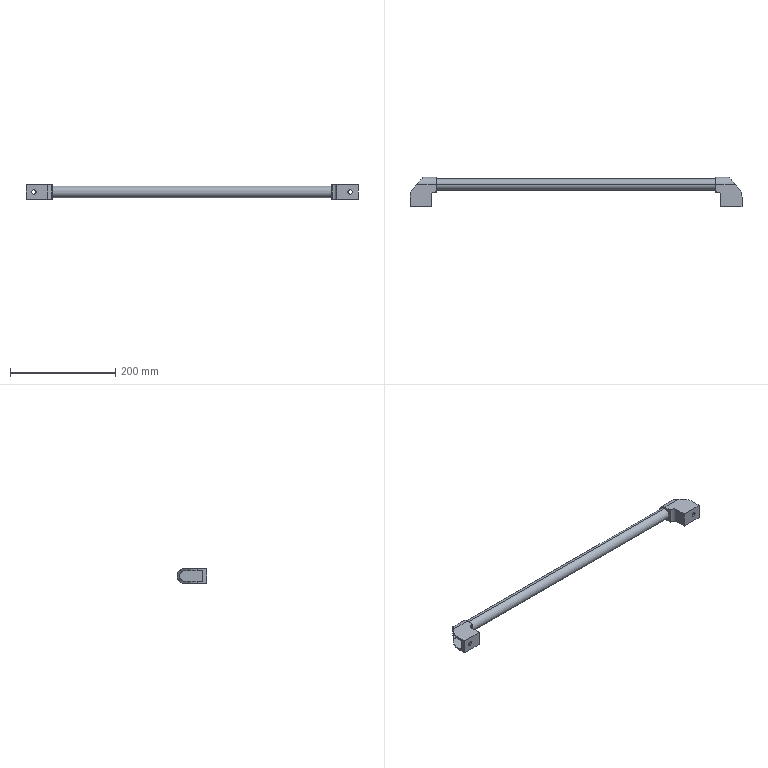Part | SolidWorks | features BaseBody 1 | 1 solid | 44 faces | box 630 x 56 x 28 mm | volume 285971 mm3 | plane 24 | cylinder 16 | cone 4 | commonest cylinder face diameters 8.2 x4 50 x4 16 x2 20 x2 22 x2 28 x2
STEP:
#1=CARTESIAN_POINT('',(265.,0.,11.));
#2=VERTEX_POINT('',#1);
#3=CARTESIAN_POINT('',(265.,0.,-11.));
#4=VERTEX_POINT('',#3);
#5=CARTESIAN_POINT('',(265.,0.,0.));
#6=DIRECTION('',(-1.,0.,0.));
#7=DIRECTION('',(0.,0.,1.));
#8=AXIS2_PLACEMENT_3D('',#5,#6,#7);
#9=CIRCLE('',#8,11.);
#10=EDGE_CURVE('',#2,#4,#9,.T.);
#11=ORIENTED_EDGE('',*,*,#10,.T.);
#12=CARTESIAN_POINT('',(-265.,0.,-11.));
#13=VERTEX_POINT('',#12);
#14=CARTESIAN_POINT('',(290.,0.,-11.));
#15=DIRECTION('',(-1.,0.,0.));
#16=VECTOR('',#15,1000.);
#17=LINE('',#14,#16);
#18=EDGE_CURVE('',#4,#13,#17,.T.);
#19=ORIENTED_EDGE('',*,*,#18,.T.);
#20=CARTESIAN_POINT('',(-265.,0.,11.));
#21=VERTEX_POINT('',#20);
#22=CARTESIAN_POINT('',(-265.,0.,0.));
#23=DIRECTION('',(1.,0.,0.));
#24=DIRECTION('',(0.,0.,1.));
#25=AXIS2_PLACEMENT_3D('',#22,#23,#24);
#26=CIRCLE('',#25,11.);
#27=EDGE_CURVE('',#13,#21,#26,.T.);
#28=ORIENTED_EDGE('',*,*,#27,.T.);
#29=CARTESIAN_POINT('',(290.,0.,11.));
#30=DIRECTION('',(-1.,0.,0.));
#31=VECTOR('',#30,1000.);
#32=LINE('',#29,#31);
#33=EDGE_CURVE('',#2,#21,#32,.T.);
#34=ORIENTED_EDGE('',*,*,#33,.F.);
#35=EDGE_LOOP('',(#11,#19,#28,#34));
#36=FACE_OUTER_BOUND('',#35,.T.);
#37=CARTESIAN_POINT('',(290.,0.,0.));
#38=DIRECTION('',(-1.,0.,0.));
#39=DIRECTION('',(0.,0.,1.));
#40=AXIS2_PLACEMENT_3D('',#37,#38,#39);
#41=CYLINDRICAL_SURFACE('',#40,11.);
#42=ADVANCED_FACE('',(#36),#41,.T.);
#43=CARTESIAN_POINT('',(-300.,-42.,4.1));
#44=VERTEX_POINT('',#43);
#45=CARTESIAN_POINT('',(-300.,-42.,-4.1));
#46=VERTEX_POINT('',#45);
#47=CARTESIAN_POINT('',(-300.,-42.,0.));
#48=DIRECTION('',(0.,-1.,0.));
#49=DIRECTION('',(0.,0.,1.));
#50=AXIS2_PLACEMENT_3D('',#47,#48,#49);
#51=CIRCLE('',#50,4.1);
#52=EDGE_CURVE('',#44,#46,#51,.T.);
#53=ORIENTED_EDGE('',*,*,#52,.T.);
#54=CARTESIAN_POINT('',(-300.,-38.,-4.1));
#55=VERTEX_POINT('',#54);
#56=CARTESIAN_POINT('',(-300.,-42.,-4.1));
#57=DIRECTION('',(0.,1.,0.));
#58=VECTOR('',#57,1000.);
#59=LINE('',#56,#58);
#60=EDGE_CURVE('',#46,#55,#59,.T.);
#61=ORIENTED_EDGE('',*,*,#60,.T.);
#62=CARTESIAN_POINT('',(-300.,-38.,4.1));
#63=VERTEX_POINT('',#62);
#64=CARTESIAN_POINT('',(-300.,-38.,0.));
#65=DIRECTION('',(0.,-1.,0.));
#66=DIRECTION('',(0.,0.,1.));
#67=AXIS2_PLACEMENT_3D('',#64,#65,#66);
#68=CIRCLE('',#67,4.1);
#69=EDGE_CURVE('',#63,#55,#68,.T.);
#70=ORIENTED_EDGE('',*,*,#69,.F.);
#71=CARTESIAN_POINT('',(-300.,-42.,4.1));
#72=DIRECTION('',(0.,1.,0.));
#73=VECTOR('',#72,1000.);
#74=LINE('',#71,#73);
#75=EDGE_CURVE('',#44,#63,#74,.T.);
#76=ORIENTED_EDGE('',*,*,#75,.F.);
#77=EDGE_LOOP('',(#53,#61,#70,#76));
#78=FACE_OUTER_BOUND('',#77,.T.);
#79=CARTESIAN_POINT('',(-300.,-42.,0.));
#80=DIRECTION('',(0.,1.,0.));
#81=DIRECTION('',(0.,0.,1.));
#82=AXIS2_PLACEMENT_3D('',#79,#80,#81);
#83=CYLINDRICAL_SURFACE('',#82,4.1);
#84=ADVANCED_FACE('',(#78),#83,.F.);
#85=CARTESIAN_POINT('',(300.,-42.,-4.1));
#86=VERTEX_POINT('',#85);
#87=CARTESIAN_POINT('',(300.,-42.,4.1));
#88=VERTEX_POINT('',#87);
#89=CARTESIAN_POINT('',(300.,-42.,0.));
#90=DIRECTION('',(0.,1.,0.));
#91=DIRECTION('',(0.,0.,1.));
#92=AXIS2_PLACEMENT_3D('',#89,#90,#91);
#93=CIRCLE('',#92,4.1);
#94=EDGE_CURVE('',#86,#88,#93,.T.);
#95=ORIENTED_EDGE('',*,*,#94,.F.);
#96=CARTESIAN_POINT('',(300.,-38.,-4.1));
#97=VERTEX_POINT('',#96);
#98=CARTESIAN_POINT('',(300.,-42.,-4.1));
#99=DIRECTION('',(0.,1.,0.));
#100=VECTOR('',#99,1000.);
#101=LINE('',#98,#100);
#102=EDGE_CURVE('',#86,#97,#101,.T.);
#103=ORIENTED_EDGE('',*,*,#102,.T.);
#104=CARTESIAN_POINT('',(300.,-38.,4.1));
#105=VERTEX_POINT('',#104);
#106=CARTESIAN_POINT('',(300.,-38.,0.));
#107=DIRECTION('',(0.,-1.,0.));
#108=DIRECTION('',(0.,0.,1.));
#109=AXIS2_PLACEMENT_3D('',#106,#107,#108);
#110=CIRCLE('',#109,4.1);
#111=EDGE_CURVE('',#105,#97,#110,.T.);
#112=ORIENTED_EDGE('',*,*,#111,.F.);
#113=CARTESIAN_POINT('',(300.,-42.,4.1));
#114=DIRECTION('',(0.,1.,0.));
#115=VECTOR('',#114,1000.);
#116=LINE('',#113,#115);
#117=EDGE_CURVE('',#88,#105,#116,.T.);
#118=ORIENTED_EDGE('',*,*,#117,.F.);
#119=EDGE_LOOP('',(#95,#103,#112,#118));
#120=FACE_OUTER_BOUND('',#119,.T.);
#121=CARTESIAN_POINT('',(300.,-42.,0.));
#122=DIRECTION('',(0.,1.,0.));
#123=DIRECTION('',(0.,0.,1.));
#124=AXIS2_PLACEMENT_3D('',#121,#122,#123);
#125=CYLINDRICAL_SURFACE('',#124,4.1);
#126=ADVANCED_FACE('',(#120),#125,.F.);
#127=ORIENTED_EDGE('',*,*,#69,.T.);
#128=CARTESIAN_POINT('',(-300.,-34.,-8.));
#129=VERTEX_POINT('',#128);
#130=CARTESIAN_POINT('',(-300.,-34.,-8.));
#131=DIRECTION('',(0.,0.716,-0.6981));
#132=VECTOR('',#131,1000.);
#133=LINE('',#130,#132);
#134=EDGE_CURVE('',#55,#129,#133,.T.);
#135=ORIENTED_EDGE('',*,*,#134,.T.);
#136=CARTESIAN_POINT('',(-300.,-34.,8.));
#137=VERTEX_POINT('',#136);
#138=CARTESIAN_POINT('',(-300.,-34.,0.));
#139=DIRECTION('',(0.,-1.,0.));
#140=DIRECTION('',(0.,0.,1.));
#141=AXIS2_PLACEMENT_3D('',#138,#139,#140);
#142=CIRCLE('',#141,8.);
#143=EDGE_CURVE('',#137,#129,#142,.T.);
#144=ORIENTED_EDGE('',*,*,#143,.F.);
#145=CARTESIAN_POINT('',(-300.,-34.,8.));
#146=DIRECTION('',(0.,0.716,0.6981));
#147=VECTOR('',#146,1000.);
#148=LINE('',#145,#147);
#149=EDGE_CURVE('',#63,#137,#148,.T.);
#150=ORIENTED_EDGE('',*,*,#149,.F.);
#151=EDGE_LOOP('',(#127,#135,#144,#150));
#152=FACE_OUTER_BOUND('',#151,.T.);
#153=CARTESIAN_POINT('',(-300.,-34.,0.));
#154=DIRECTION('',(0.,1.,0.));
#155=DIRECTION('',(0.,0.,1.));
#156=AXIS2_PLACEMENT_3D('',#153,#154,#155);
#157=CONICAL_SURFACE('',#156,8.,0.7727);
#158=ADVANCED_FACE('',(#152),#157,.F.);
#159=ORIENTED_EDGE('',*,*,#111,.T.);
#160=CARTESIAN_POINT('',(300.,-34.,-8.));
#161=VERTEX_POINT('',#160);
#162=CARTESIAN_POINT('',(300.,-34.,-8.));
#163=DIRECTION('',(0.,0.716,-0.6981));
#164=VECTOR('',#163,1000.);
#165=LINE('',#162,#164);
#166=EDGE_CURVE('',#97,#161,#165,.T.);
#167=ORIENTED_EDGE('',*,*,#166,.T.);
#168=CARTESIAN_POINT('',(300.,-34.,8.));
#169=VERTEX_POINT('',#168);
#170=CARTESIAN_POINT('',(300.,-34.,0.));
#171=DIRECTION('',(0.,1.,0.));
#172=DIRECTION('',(0.,0.,1.));
#173=AXIS2_PLACEMENT_3D('',#170,#171,#172);
#174=CIRCLE('',#173,8.);
#175=EDGE_CURVE('',#161,#169,#174,.T.);
#176=ORIENTED_EDGE('',*,*,#175,.T.);
#177=CARTESIAN_POINT('',(300.,-34.,8.));
#178=DIRECTION('',(0.,0.716,0.6981));
#179=VECTOR('',#178,1000.);
#180=LINE('',#177,#179);
#181=EDGE_CURVE('',#105,#169,#180,.T.);
#182=ORIENTED_EDGE('',*,*,#181,.F.);
#183=EDGE_LOOP('',(#159,#167,#176,#182));
#184=FACE_OUTER_BOUND('',#183,.T.);
#185=CARTESIAN_POINT('',(300.,-34.,0.));
#186=DIRECTION('',(0.,1.,0.));
#187=DIRECTION('',(0.,0.,1.));
#188=AXIS2_PLACEMENT_3D('',#185,#186,#187);
#189=CONICAL_SURFACE('',#188,8.,0.7727);
#190=ADVANCED_FACE('',(#184),#189,.F.);
#191=ORIENTED_EDGE('',*,*,#18,.F.);
#192=CARTESIAN_POINT('',(265.,0.,0.));
#193=DIRECTION('',(-1.,0.,0.));
#194=DIRECTION('',(0.,0.,1.));
#195=AXIS2_PLACEMENT_3D('',#192,#193,#194);
#196=CIRCLE('',#195,11.);
#197=EDGE_CURVE('',#4,#2,#196,.T.);
#198=ORIENTED_EDGE('',*,*,#197,.T.);
#199=ORIENTED_EDGE('',*,*,#33,.T.);
#200=CARTESIAN_POINT('',(-265.,0.,0.));
#201=DIRECTION('',(1.,0.,0.));
#202=DIRECTION('',(0.,0.,1.));
#203=AXIS2_PLACEMENT_3D('',#200,#201,#202);
#204=CIRCLE('',#203,11.);
#205=EDGE_CURVE('',#21,#13,#204,.T.);
#206=ORIENTED_EDGE('',*,*,#205,.T.);
#207=EDGE_LOOP('',(#191,#198,#199,#206));
#208=FACE_OUTER_BOUND('',#207,.T.);
#209=CARTESIAN_POINT('',(290.,0.,0.));
#210=DIRECTION('',(-1.,0.,0.));
#211=DIRECTION('',(0.,0.,1.));
#212=AXIS2_PLACEMENT_3D('',#209,#210,#211);
#213=CYLINDRICAL_SURFACE('',#212,11.);
#214=ADVANCED_FACE('',(#208),#213,.T.);
#215=ORIENTED_EDGE('',*,*,#205,.F.);
#216=ORIENTED_EDGE('',*,*,#27,.F.);
#217=EDGE_LOOP('',(#215,#216));
#218=FACE_BOUND('',#217,.T.);
#219=CARTESIAN_POINT('',(-265.,0.,-14.));
#220=VERTEX_POINT('',#219);
#221=CARTESIAN_POINT('',(-265.,-14.,-14.));
#222=VERTEX_POINT('',#221);
#223=CARTESIAN_POINT('',(-265.,-14.,-14.));
#224=DIRECTION('',(0.,-1.,0.));
#225=VECTOR('',#224,1000.);
#226=LINE('',#223,#225);
#227=EDGE_CURVE('',#220,#222,#226,.T.);
#228=ORIENTED_EDGE('',*,*,#227,.F.);
#229=CARTESIAN_POINT('',(-265.,0.000000104,14.));
#230=VERTEX_POINT('',#229);
#231=CARTESIAN_POINT('',(-265.,0.,0.));
#232=DIRECTION('',(-1.,0.,0.));
#233=DIRECTION('',(0.,0.,-1.));
#234=AXIS2_PLACEMENT_3D('',#231,#232,#233);
#235=CIRCLE('',#234,14.);
#236=EDGE_CURVE('',#230,#220,#235,.T.);
#237=ORIENTED_EDGE('',*,*,#236,.F.);
#238=CARTESIAN_POINT('',(-265.,-14.,14.));
#239=VERTEX_POINT('',#238);
#240=CARTESIAN_POINT('',(-265.,-14.,14.));
#241=DIRECTION('',(0.,1.,0.));
#242=VECTOR('',#241,1000.);
#243=LINE('',#240,#242);
#244=EDGE_CURVE('',#239,#230,#243,.T.);
#245=ORIENTED_EDGE('',*,*,#244,.F.);
#246=CARTESIAN_POINT('',(-265.,-14.,28.));
#247=DIRECTION('',(0.,0.,1.));
#248=VECTOR('',#247,1000.);
#249=LINE('',#246,#248);
#250=EDGE_CURVE('',#222,#239,#249,.T.);
#251=ORIENTED_EDGE('',*,*,#250,.F.);
#252=EDGE_LOOP('',(#228,#237,#245,#251));
#253=FACE_OUTER_BOUND('',#252,.T.);
#254=CARTESIAN_POINT('',(-265.,-14.,28.));
#255=DIRECTION('',(-1.,0.,0.));
#256=DIRECTION('',(0.,0.,1.));
#257=AXIS2_PLACEMENT_3D('',#254,#255,#256);
#258=PLANE('',#257);
#259=ADVANCED_FACE('',(#218,#253),#258,.F.);
#260=CARTESIAN_POINT('',(265.,0.000000104,14.));
#261=VERTEX_POINT('',#260);
#262=CARTESIAN_POINT('',(265.,-14.,14.));
#263=VERTEX_POINT('',#262);
#264=CARTESIAN_POINT('',(265.,0.,14.));
#265=DIRECTION('',(0.,-1.,0.));
#266=VECTOR('',#265,1000.);
#267=LINE('',#264,#266);
#268=EDGE_CURVE('',#261,#263,#267,.T.);
#269=ORIENTED_EDGE('',*,*,#268,.F.);
#270=CARTESIAN_POINT('',(265.,0.,-14.));
#271=VERTEX_POINT('',#270);
#272=CARTESIAN_POINT('',(265.,0.,0.));
#273=DIRECTION('',(1.,0.,0.));
#274=DIRECTION('',(0.,0.,1.));
#275=AXIS2_PLACEMENT_3D('',#272,#273,#274);
#276=CIRCLE('',#275,14.);
#277=EDGE_CURVE('',#271,#261,#276,.T.);
#278=ORIENTED_EDGE('',*,*,#277,.F.);
#279=CARTESIAN_POINT('',(265.,-14.,-14.));
#280=VERTEX_POINT('',#279);
#281=CARTESIAN_POINT('',(265.,0.,-14.));
#282=DIRECTION('',(0.,1.,0.));
#283=VECTOR('',#282,1000.);
#284=LINE('',#281,#283);
#285=EDGE_CURVE('',#280,#271,#284,.T.);
#286=ORIENTED_EDGE('',*,*,#285,.F.);
#287=CARTESIAN_POINT('',(265.,-14.,0.));
#288=DIRECTION('',(0.,0.,-1.));
#289=VECTOR('',#288,1000.);
#290=LINE('',#287,#289);
#291=EDGE_CURVE('',#263,#280,#290,.T.);
#292=ORIENTED_EDGE('',*,*,#291,.F.);
#293=EDGE_LOOP('',(#269,#278,#286,#292));
#294=FACE_OUTER_BOUND('',#293,.T.);
#295=ORIENTED_EDGE('',*,*,#10,.F.);
#296=ORIENTED_EDGE('',*,*,#197,.F.);
#297=EDGE_LOOP('',(#295,#296));
#298=FACE_BOUND('',#297,.T.);
#299=CARTESIAN_POINT('',(265.,0.,0.));
#300=DIRECTION('',(1.,0.,0.));
#301=DIRECTION('',(0.,0.,-1.));
#302=AXIS2_PLACEMENT_3D('',#299,#300,#301);
#303=PLANE('',#302);
#304=ADVANCED_FACE('',(#294,#298),#303,.F.);
#305=CARTESIAN_POINT('',(-267.,-14.,-14.));
#306=VERTEX_POINT('',#305);
#307=CARTESIAN_POINT('',(-267.,-14.,-14.));
#308=DIRECTION('',(-1.,0.,0.));
#309=VECTOR('',#308,1000.);
#310=LINE('',#307,#309);
#311=EDGE_CURVE('',#222,#306,#310,.T.);
#312=ORIENTED_EDGE('',*,*,#311,.F.);
#313=ORIENTED_EDGE('',*,*,#250,.T.);
#314=CARTESIAN_POINT('',(-267.,-14.,14.));
#315=VERTEX_POINT('',#314);
#316=CARTESIAN_POINT('',(-267.,-14.,14.));
#317=DIRECTION('',(1.,0.,0.));
#318=VECTOR('',#317,1000.);
#319=LINE('',#316,#318);
#320=EDGE_CURVE('',#315,#239,#319,.T.);
#321=ORIENTED_EDGE('',*,*,#320,.F.);
#322=CARTESIAN_POINT('',(-267.,-14.,28.));
#323=DIRECTION('',(0.,0.,1.));
#324=VECTOR('',#323,1000.);
#325=LINE('',#322,#324);
#326=EDGE_CURVE('',#306,#315,#325,.T.);
#327=ORIENTED_EDGE('',*,*,#326,.F.);
#328=EDGE_LOOP('',(#312,#313,#321,#327));
#329=FACE_OUTER_BOUND('',#328,.T.);
#330=CARTESIAN_POINT('',(-267.,-14.,28.));
#331=DIRECTION('',(0.,1.,0.));
#332=DIRECTION('',(0.,0.,1.));
#333=AXIS2_PLACEMENT_3D('',#330,#331,#332);
#334=PLANE('',#333);
#335=ADVANCED_FACE('',(#329),#334,.F.);
#336=CARTESIAN_POINT('',(-308.648,-6.886,-14.));
#337=VERTEX_POINT('',#336);
#338=CARTESIAN_POINT('',(-315.,-23.537,-14.));
#339=VERTEX_POINT('',#338);
#340=CARTESIAN_POINT('',(-290.,-23.537,-14.));
#341=DIRECTION('',(0.,0.,1.));
#342=DIRECTION('',(1.,0.,0.));
#343=AXIS2_PLACEMENT_3D('',#340,#341,#342);
#344=CIRCLE('',#343,25.);
#345=EDGE_CURVE('',#337,#339,#344,.T.);
#346=ORIENTED_EDGE('',*,*,#345,.F.);
#347=CARTESIAN_POINT('',(-302.5,0.,-14.));
#348=VERTEX_POINT('',#347);
#349=CARTESIAN_POINT('',(-302.5,0.,-14.));
#350=DIRECTION('',(-0.666,-0.7459,0.));
#351=VECTOR('',#350,1000.);
#352=LINE('',#349,#351);
#353=EDGE_CURVE('',#348,#337,#352,.T.);
#354=ORIENTED_EDGE('',*,*,#353,.F.);
#355=CARTESIAN_POINT('',(315.,0.,-14.));
#356=DIRECTION('',(-1.,0.,0.));
#357=VECTOR('',#356,1000.);
#358=LINE('',#355,#357);
#359=EDGE_CURVE('',#220,#348,#358,.T.);
#360=ORIENTED_EDGE('',*,*,#359,.F.);
#361=ORIENTED_EDGE('',*,*,#227,.T.);
#362=ORIENTED_EDGE('',*,*,#311,.T.);
#363=CARTESIAN_POINT('',(-275.,-22.,-14.));
#364=VERTEX_POINT('',#363);
#365=CARTESIAN_POINT('',(-267.,-22.,-14.));
#366=DIRECTION('',(0.,0.,-1.));
#367=DIRECTION('',(1.,0.,0.));
#368=AXIS2_PLACEMENT_3D('',#365,#366,#367);
#369=CIRCLE('',#368,8.);
#370=EDGE_CURVE('',#364,#306,#369,.T.);
#371=ORIENTED_EDGE('',*,*,#370,.F.);
#372=CARTESIAN_POINT('',(-275.,-42.,-14.));
#373=VERTEX_POINT('',#372);
#374=CARTESIAN_POINT('',(-275.,-42.,-14.));
#375=DIRECTION('',(0.,1.,0.));
#376=VECTOR('',#375,1000.);
#377=LINE('',#374,#376);
#378=EDGE_CURVE('',#373,#364,#377,.T.);
#379=ORIENTED_EDGE('',*,*,#378,.F.);
#380=CARTESIAN_POINT('',(-315.,-42.,-14.));
#381=VERTEX_POINT('',#380);
#382=CARTESIAN_POINT('',(315.,-42.,-14.));
#383=DIRECTION('',(1.,0.,0.));
#384=VECTOR('',#383,1000.);
#385=LINE('',#382,#384);
#386=EDGE_CURVE('',#381,#373,#385,.T.);
#387=ORIENTED_EDGE('',*,*,#386,.F.);
#388=CARTESIAN_POINT('',(-315.,-42.,-14.));
#389=DIRECTION('',(0.,-1.,0.));
#390=VECTOR('',#389,1000.);
#391=LINE('',#388,#390);
#392=EDGE_CURVE('',#339,#381,#391,.T.);
#393=ORIENTED_EDGE('',*,*,#392,.F.);
#394=EDGE_LOOP('',(#346,#354,#360,#361,#362,#371,#379,#387,#393));
#395=FACE_OUTER_BOUND('',#394,.T.);
#396=CARTESIAN_POINT('',(315.,-42.,-14.));
#397=DIRECTION('',(0.,0.,1.));
#398=DIRECTION('',(1.,0.,0.));
#399=AXIS2_PLACEMENT_3D('',#396,#397,#398);
#400=PLANE('',#399);
#401=ADVANCED_FACE('',(#395),#400,.F.);
#402=CARTESIAN_POINT('',(-302.5,0.000000104,14.));
#403=VERTEX_POINT('',#402);
#404=CARTESIAN_POINT('',(-302.5,0.,-14.));
#405=CARTESIAN_POINT('',(-277.5,28.,-14.));
#406=CARTESIAN_POINT('',(-277.5,28.,14.));
#407=CARTESIAN_POINT('',(-302.5,0.000000104,14.));
#408=(BOUNDED_CURVE()B_SPLINE_CURVE(3,(#404,#405,#406,#407),.UNSPECIFIED.,.F.,.T.)B_SPLINE_CURVE_WITH_KNOTS((4,4),(4.712,7.854),.UNSPECIFIED.)CURVE()GEOMETRIC_REPRESENTATION_ITEM()RATIONAL_B_SPLINE_CURVE((1.,0.3333,0.3333,1.))REPRESENTATION_ITEM(''));
#409=EDGE_CURVE('',#348,#403,#408,.T.);
#410=ORIENTED_EDGE('',*,*,#409,.T.);
#411=CARTESIAN_POINT('',(315.,0.000000209,14.));
#412=DIRECTION('',(1.,0.,0.));
#413=VECTOR('',#412,1000.);
#414=LINE('',#411,#413);
#415=EDGE_CURVE('',#403,#230,#414,.T.);
#416=ORIENTED_EDGE('',*,*,#415,.T.);
#417=ORIENTED_EDGE('',*,*,#236,.T.);
#418=ORIENTED_EDGE('',*,*,#359,.T.);
#419=EDGE_LOOP('',(#410,#416,#417,#418));
#420=FACE_OUTER_BOUND('',#419,.T.);
#421=CARTESIAN_POINT('',(315.,0.,0.));
#422=DIRECTION('',(1.,0.,0.));
#423=DIRECTION('',(0.,0.,-1.));
#424=AXIS2_PLACEMENT_3D('',#421,#422,#423);
#425=CYLINDRICAL_SURFACE('',#424,14.);
#426=ADVANCED_FACE('',(#420),#425,.T.);
#427=CARTESIAN_POINT('',(-315.,-23.537,14.));
#428=VERTEX_POINT('',#427);
#429=CARTESIAN_POINT('',(-308.648,-6.886,14.));
#430=VERTEX_POINT('',#429);
#431=CARTESIAN_POINT('',(-290.,-23.537,14.));
#432=DIRECTION('',(0.,0.,-1.));
#433=DIRECTION('',(1.,0.,0.));
#434=AXIS2_PLACEMENT_3D('',#431,#432,#433);
#435=CIRCLE('',#434,25.);
#436=EDGE_CURVE('',#428,#430,#435,.T.);
#437=ORIENTED_EDGE('',*,*,#436,.F.);
#438=CARTESIAN_POINT('',(-315.,-42.,14.));
#439=VERTEX_POINT('',#438);
#440=CARTESIAN_POINT('',(-315.,0.,14.));
#441=DIRECTION('',(0.,1.,0.));
#442=VECTOR('',#441,1000.);
#443=LINE('',#440,#442);
#444=EDGE_CURVE('',#439,#428,#443,.T.);
#445=ORIENTED_EDGE('',*,*,#444,.F.);
#446=CARTESIAN_POINT('',(-275.,-42.,14.));
#447=VERTEX_POINT('',#446);
#448=CARTESIAN_POINT('',(315.,-42.,14.));
#449=DIRECTION('',(-1.,0.,0.));
#450=VECTOR('',#449,1000.);
#451=LINE('',#448,#450);
#452=EDGE_CURVE('',#447,#439,#451,.T.);
#453=ORIENTED_EDGE('',*,*,#452,.F.);
#454=CARTESIAN_POINT('',(-275.,-22.,14.));
#455=VERTEX_POINT('',#454);
#456=CARTESIAN_POINT('',(-275.,0.,14.));
#457=DIRECTION('',(0.,-1.,0.));
#458=VECTOR('',#457,1000.);
#459=LINE('',#456,#458);
#460=EDGE_CURVE('',#455,#447,#459,.T.);
#461=ORIENTED_EDGE('',*,*,#460,.F.);
#462=CARTESIAN_POINT('',(-267.,-22.,14.));
#463=DIRECTION('',(0.,0.,1.));
#464=DIRECTION('',(1.,0.,0.));
#465=AXIS2_PLACEMENT_3D('',#462,#463,#464);
#466=CIRCLE('',#465,8.);
#467=EDGE_CURVE('',#315,#455,#466,.T.);
#468=ORIENTED_EDGE('',*,*,#467,.F.);
#469=ORIENTED_EDGE('',*,*,#320,.T.);
#470=ORIENTED_EDGE('',*,*,#244,.T.);
#471=ORIENTED_EDGE('',*,*,#415,.F.);
#472=CARTESIAN_POINT('',(-308.648,-6.886,14.));
#473=DIRECTION('',(0.666,0.7459,0.));
#474=VECTOR('',#473,1000.);
#475=LINE('',#472,#474);
#476=EDGE_CURVE('',#430,#403,#475,.T.);
#477=ORIENTED_EDGE('',*,*,#476,.F.);
#478=EDGE_LOOP('',(#437,#445,#453,#461,#468,#469,#470,#471,#477));
#479=FACE_OUTER_BOUND('',#478,.T.);
#480=CARTESIAN_POINT('',(315.,0.,14.));
#481=DIRECTION('',(0.,0.,-1.));
#482=DIRECTION('',(-1.,0.,0.));
#483=AXIS2_PLACEMENT_3D('',#480,#481,#482);
#484=PLANE('',#483);
#485=ADVANCED_FACE('',(#479),#484,.F.);
#486=CARTESIAN_POINT('',(267.,-14.,-14.));
#487=VERTEX_POINT('',#486);
#488=CARTESIAN_POINT('',(267.,-14.,14.));
#489=VERTEX_POINT('',#488);
#490=CARTESIAN_POINT('',(267.,-14.,28.));
#491=DIRECTION('',(0.,0.,1.));
#492=VECTOR('',#491,1000.);
#493=LINE('',#490,#492);
#494=EDGE_CURVE('',#487,#489,#493,.T.);
#495=ORIENTED_EDGE('',*,*,#494,.T.);
#496=CARTESIAN_POINT('',(267.,-14.,14.));
#497=DIRECTION('',(-1.,0.,0.));
#498=VECTOR('',#497,1000.);
#499=LINE('',#496,#498);
#500=EDGE_CURVE('',#489,#263,#499,.T.);
#501=ORIENTED_EDGE('',*,*,#500,.T.);
#502=ORIENTED_EDGE('',*,*,#291,.T.);
#503=CARTESIAN_POINT('',(267.,-14.,-14.));
#504=DIRECTION('',(1.,0.,0.));
#505=VECTOR('',#504,1000.);
#506=LINE('',#503,#505);
#507=EDGE_CURVE('',#280,#487,#506,.T.);
#508=ORIENTED_EDGE('',*,*,#507,.T.);
#509=EDGE_LOOP('',(#495,#501,#502,#508));
#510=FACE_OUTER_BOUND('',#509,.T.);
#511=CARTESIAN_POINT('',(267.,-14.,28.));
#512=DIRECTION('',(0.,-1.,0.));
#513=DIRECTION('',(0.,0.,-1.));
#514=AXIS2_PLACEMENT_3D('',#511,#512,#513);
#515=PLANE('',#514);
#516=ADVANCED_FACE('',(#510),#515,.T.);
#517=CARTESIAN_POINT('',(275.,-42.,14.));
#518=VERTEX_POINT('',#517);
#519=CARTESIAN_POINT('',(315.,-42.,14.));
#520=VERTEX_POINT('',#519);
#521=CARTESIAN_POINT('',(265.,-42.,14.));
#522=DIRECTION('',(1.,0.,0.));
#523=VECTOR('',#522,1000.);
#524=LINE('',#521,#523);
#525=EDGE_CURVE('',#518,#520,#524,.T.);
#526=ORIENTED_EDGE('',*,*,#525,.T.);
#527=CARTESIAN_POINT('',(315.,-23.537,14.));
#528=VERTEX_POINT('',#527);
#529=CARTESIAN_POINT('',(315.,0.,14.));
#530=DIRECTION('',(0.,1.,0.));
#531=VECTOR('',#530,1000.);
#532=LINE('',#529,#531);
#533=EDGE_CURVE('',#520,#528,#532,.T.);
#534=ORIENTED_EDGE('',*,*,#533,.T.);
#535=CARTESIAN_POINT('',(308.648,-6.886,14.));
#536=VERTEX_POINT('',#535);
#537=CARTESIAN_POINT('',(290.,-23.537,14.));
#538=DIRECTION('',(0.,0.,1.));
#539=DIRECTION('',(1.,0.,0.));
#540=AXIS2_PLACEMENT_3D('',#537,#538,#539);
#541=CIRCLE('',#540,25.);
#542=EDGE_CURVE('',#528,#536,#541,.T.);
#543=ORIENTED_EDGE('',*,*,#542,.T.);
#544=CARTESIAN_POINT('',(302.5,0.000000104,14.));
#545=VERTEX_POINT('',#544);
#546=CARTESIAN_POINT('',(308.648,-6.886,14.));
#547=DIRECTION('',(-0.666,0.7459,0.));
#548=VECTOR('',#547,1000.);
#549=LINE('',#546,#548);
#550=EDGE_CURVE('',#536,#545,#549,.T.);
#551=ORIENTED_EDGE('',*,*,#550,.T.);
#552=CARTESIAN_POINT('',(265.,0.000000209,14.));
#553=DIRECTION('',(-1.,0.,0.));
#554=VECTOR('',#553,1000.);
#555=LINE('',#552,#554);
#556=EDGE_CURVE('',#545,#261,#555,.T.);
#557=ORIENTED_EDGE('',*,*,#556,.T.);
#558=ORIENTED_EDGE('',*,*,#268,.T.);
#559=ORIENTED_EDGE('',*,*,#500,.F.);
#560=CARTESIAN_POINT('',(275.,-22.,14.));
#561=VERTEX_POINT('',#560);
#562=CARTESIAN_POINT('',(267.,-22.,14.));
#563=DIRECTION('',(0.,0.,-1.));
#564=DIRECTION('',(1.,0.,0.));
#565=AXIS2_PLACEMENT_3D('',#562,#563,#564);
#566=CIRCLE('',#565,8.);
#567=EDGE_CURVE('',#489,#561,#566,.T.);
#568=ORIENTED_EDGE('',*,*,#567,.T.);
#569=CARTESIAN_POINT('',(275.,0.,14.));
#570=DIRECTION('',(0.,-1.,0.));
#571=VECTOR('',#570,1000.);
#572=LINE('',#569,#571);
#573=EDGE_CURVE('',#561,#518,#572,.T.);
#574=ORIENTED_EDGE('',*,*,#573,.T.);
#575=EDGE_LOOP('',(#526,#534,#543,#551,#557,#558,#559,#568,#574));
#576=FACE_OUTER_BOUND('',#575,.T.);
#577=CARTESIAN_POINT('',(265.,0.,14.));
#578=DIRECTION('',(0.,0.,1.));
#579=DIRECTION('',(1.,0.,0.));
#580=AXIS2_PLACEMENT_3D('',#577,#578,#579);
#581=PLANE('',#580);
#582=ADVANCED_FACE('',(#576),#581,.T.);
#583=CARTESIAN_POINT('',(302.5,0.,-14.));
#584=VERTEX_POINT('',#583);
#585=CARTESIAN_POINT('',(265.,0.,-14.));
#586=DIRECTION('',(-1.,0.,0.));
#587=VECTOR('',#586,1000.);
#588=LINE('',#585,#587);
#589=EDGE_CURVE('',#584,#271,#588,.T.);
#590=ORIENTED_EDGE('',*,*,#589,.T.);
#591=ORIENTED_EDGE('',*,*,#277,.T.);
#592=ORIENTED_EDGE('',*,*,#556,.F.);
#593=CARTESIAN_POINT('',(302.5,0.000000104,14.));
#594=CARTESIAN_POINT('',(277.5,28.,14.));
#595=CARTESIAN_POINT('',(277.5,28.,-14.));
#596=CARTESIAN_POINT('',(302.5,0.,-14.));
#597=(BOUNDED_CURVE()B_SPLINE_CURVE(3,(#593,#594,#595,#596),.UNSPECIFIED.,.F.,.F.)B_SPLINE_CURVE_WITH_KNOTS((4,4),(4.712,7.854),.UNSPECIFIED.)CURVE()GEOMETRIC_REPRESENTATION_ITEM()RATIONAL_B_SPLINE_CURVE((1.,0.3333,0.3333,1.))REPRESENTATION_ITEM(''));
#598=EDGE_CURVE('',#545,#584,#597,.T.);
#599=ORIENTED_EDGE('',*,*,#598,.T.);
#600=EDGE_LOOP('',(#590,#591,#592,#599));
#601=FACE_OUTER_BOUND('',#600,.T.);
#602=CARTESIAN_POINT('',(265.,0.,0.));
#603=DIRECTION('',(-1.,0.,0.));
#604=DIRECTION('',(0.,0.,1.));
#605=AXIS2_PLACEMENT_3D('',#602,#603,#604);
#606=CYLINDRICAL_SURFACE('',#605,14.);
#607=ADVANCED_FACE('',(#601),#606,.T.);
#608=ORIENTED_EDGE('',*,*,#507,.F.);
#609=ORIENTED_EDGE('',*,*,#285,.T.);
#610=ORIENTED_EDGE('',*,*,#589,.F.);
#611=CARTESIAN_POINT('',(308.648,-6.886,-14.));
#612=VERTEX_POINT('',#611);
#613=CARTESIAN_POINT('',(302.5,0.,-14.));
#614=DIRECTION('',(0.666,-0.7459,0.));
#615=VECTOR('',#614,1000.);
#616=LINE('',#613,#615);
#617=EDGE_CURVE('',#584,#612,#616,.T.);
#618=ORIENTED_EDGE('',*,*,#617,.T.);
#619=CARTESIAN_POINT('',(315.,-23.537,-14.));
#620=VERTEX_POINT('',#619);
#621=CARTESIAN_POINT('',(290.,-23.537,-14.));
#622=DIRECTION('',(0.,0.,-1.));
#623=DIRECTION('',(1.,0.,0.));
#624=AXIS2_PLACEMENT_3D('',#621,#622,#623);
#625=CIRCLE('',#624,25.);
#626=EDGE_CURVE('',#612,#620,#625,.T.);
#627=ORIENTED_EDGE('',*,*,#626,.T.);
#628=CARTESIAN_POINT('',(315.,-42.,-14.));
#629=VERTEX_POINT('',#628);
#630=CARTESIAN_POINT('',(315.,-42.,-14.));
#631=DIRECTION('',(0.,-1.,0.));
#632=VECTOR('',#631,1000.);
#633=LINE('',#630,#632);
#634=EDGE_CURVE('',#620,#629,#633,.T.);
#635=ORIENTED_EDGE('',*,*,#634,.T.);
#636=CARTESIAN_POINT('',(275.,-42.,-14.));
#637=VERTEX_POINT('',#636);
#638=CARTESIAN_POINT('',(265.,-42.,-14.));
#639=DIRECTION('',(-1.,0.,0.));
#640=VECTOR('',#639,1000.);
#641=LINE('',#638,#640);
#642=EDGE_CURVE('',#629,#637,#641,.T.);
#643=ORIENTED_EDGE('',*,*,#642,.T.);
#644=CARTESIAN_POINT('',(275.,-22.,-14.));
#645=VERTEX_POINT('',#644);
#646=CARTESIAN_POINT('',(275.,-42.,-14.));
#647=DIRECTION('',(0.,1.,0.));
#648=VECTOR('',#647,1000.);
#649=LINE('',#646,#648);
#650=EDGE_CURVE('',#637,#645,#649,.T.);
#651=ORIENTED_EDGE('',*,*,#650,.T.);
#652=CARTESIAN_POINT('',(267.,-22.,-14.));
#653=DIRECTION('',(0.,0.,1.));
#654=DIRECTION('',(1.,0.,0.));
#655=AXIS2_PLACEMENT_3D('',#652,#653,#654);
#656=CIRCLE('',#655,8.);
#657=EDGE_CURVE('',#645,#487,#656,.T.);
#658=ORIENTED_EDGE('',*,*,#657,.T.);
#659=EDGE_LOOP('',(#608,#609,#610,#618,#627,#635,#643,#651,#658));
#660=FACE_OUTER_BOUND('',#659,.T.);
#661=CARTESIAN_POINT('',(265.,-42.,-14.));
#662=DIRECTION('',(0.,0.,-1.));
#663=DIRECTION('',(-1.,0.,0.));
#664=AXIS2_PLACEMENT_3D('',#661,#662,#663);
#665=PLANE('',#664);
#666=ADVANCED_FACE('',(#660),#665,.T.);
#667=CARTESIAN_POINT('',(-275.,-22.,28.));
#668=DIRECTION('',(0.,0.,1.));
#669=VECTOR('',#668,1000.);
#670=LINE('',#667,#669);
#671=EDGE_CURVE('',#364,#455,#670,.T.);
#672=ORIENTED_EDGE('',*,*,#671,.F.);
#673=ORIENTED_EDGE('',*,*,#370,.T.);
#674=ORIENTED_EDGE('',*,*,#326,.T.);
#675=ORIENTED_EDGE('',*,*,#467,.T.);
#676=EDGE_LOOP('',(#672,#673,#674,#675));
#677=FACE_OUTER_BOUND('',#676,.T.);
#678=CARTESIAN_POINT('',(-267.,-22.,28.));
#679=DIRECTION('',(0.,0.,1.));
#680=DIRECTION('',(1.,0.,0.));
#681=AXIS2_PLACEMENT_3D('',#678,#679,#680);
#682=CYLINDRICAL_SURFACE('',#681,8.);
#683=ADVANCED_FACE('',(#677),#682,.F.);
#684=CARTESIAN_POINT('',(-315.,-34.,-10.));
#685=VERTEX_POINT('',#684);
#686=CARTESIAN_POINT('',(-315.,-34.,10.));
#687=VERTEX_POINT('',#686);
#688=CARTESIAN_POINT('',(-315.,-34.,0.));
#689=DIRECTION('',(0.,0.,1.));
#690=VECTOR('',#689,1000.);
#691=LINE('',#688,#690);
#692=EDGE_CURVE('',#685,#687,#691,.T.);
#693=ORIENTED_EDGE('',*,*,#692,.F.);
#694=CARTESIAN_POINT('',(-315.,-23.537,-10.));
#695=VERTEX_POINT('',#694);
#696=CARTESIAN_POINT('',(-315.,0.,-10.));
#697=DIRECTION('',(0.,-1.,0.));
#698=VECTOR('',#697,1000.);
#699=LINE('',#696,#698);
#700=EDGE_CURVE('',#695,#685,#699,.T.);
#701=ORIENTED_EDGE('',*,*,#700,.F.);
#702=CARTESIAN_POINT('',(-315.,-23.537,0.));
#703=DIRECTION('',(0.,0.,1.));
#704=VECTOR('',#703,1000.);
#705=LINE('',#702,#704);
#706=EDGE_CURVE('',#339,#695,#705,.T.);
#707=ORIENTED_EDGE('',*,*,#706,.F.);
#708=ORIENTED_EDGE('',*,*,#392,.T.);
#709=CARTESIAN_POINT('',(-315.,-42.,0.));
#710=DIRECTION('',(0.,0.,-1.));
#711=VECTOR('',#710,1000.);
#712=LINE('',#709,#711);
#713=EDGE_CURVE('',#439,#381,#712,.T.);
#714=ORIENTED_EDGE('',*,*,#713,.F.);
#715=ORIENTED_EDGE('',*,*,#444,.T.);
#716=CARTESIAN_POINT('',(-315.,-23.537,10.));
#717=VERTEX_POINT('',#716);
#718=CARTESIAN_POINT('',(-315.,-23.537,0.));
#719=DIRECTION('',(0.,0.,1.));
#720=VECTOR('',#719,1000.);
#721=LINE('',#718,#720);
#722=EDGE_CURVE('',#717,#428,#721,.T.);
#723=ORIENTED_EDGE('',*,*,#722,.F.);
#724=CARTESIAN_POINT('',(-315.,0.,10.));
#725=DIRECTION('',(0.,1.,0.));
#726=VECTOR('',#725,1000.);
#727=LINE('',#724,#726);
#728=EDGE_CURVE('',#687,#717,#727,.T.);
#729=ORIENTED_EDGE('',*,*,#728,.F.);
#730=EDGE_LOOP('',(#693,#701,#707,#708,#714,#715,#723,#729));
#731=FACE_OUTER_BOUND('',#730,.T.);
#732=CARTESIAN_POINT('',(-315.,0.,0.));
#733=DIRECTION('',(1.,0.,0.));
#734=DIRECTION('',(0.,0.,-1.));
#735=AXIS2_PLACEMENT_3D('',#732,#733,#734);
#736=PLANE('',#735);
#737=ADVANCED_FACE('',(#731),#736,.F.);
#738=ORIENTED_EDGE('',*,*,#345,.T.);
#739=ORIENTED_EDGE('',*,*,#706,.T.);
#740=CARTESIAN_POINT('',(-308.648,-6.886,-10.));
#741=VERTEX_POINT('',#740);
#742=CARTESIAN_POINT('',(-290.,-23.537,-10.));
#743=DIRECTION('',(0.,0.,-1.));
#744=DIRECTION('',(1.,0.,0.));
#745=AXIS2_PLACEMENT_3D('',#742,#743,#744);
#746=CIRCLE('',#745,25.);
#747=EDGE_CURVE('',#695,#741,#746,.T.);
#748=ORIENTED_EDGE('',*,*,#747,.T.);
#749=CARTESIAN_POINT('',(-308.648,-6.886,28.));
#750=DIRECTION('',(0.,0.,-1.));
#751=VECTOR('',#750,1000.);
#752=LINE('',#749,#751);
#753=EDGE_CURVE('',#741,#337,#752,.T.);
#754=ORIENTED_EDGE('',*,*,#753,.T.);
#755=EDGE_LOOP('',(#738,#739,#748,#754));
#756=FACE_OUTER_BOUND('',#755,.T.);
#757=CARTESIAN_POINT('',(-290.,-23.537,28.));
#758=DIRECTION('',(0.,0.,1.));
#759=DIRECTION('',(1.,0.,0.));
#760=AXIS2_PLACEMENT_3D('',#757,#758,#759);
#761=CYLINDRICAL_SURFACE('',#760,25.);
#762=ADVANCED_FACE('',(#756),#761,.T.);
#763=CARTESIAN_POINT('',(-308.648,-6.886,10.));
#764=VERTEX_POINT('',#763);
#765=CARTESIAN_POINT('',(-308.648,-6.886,28.));
#766=DIRECTION('',(0.,0.,-1.));
#767=VECTOR('',#766,1000.);
#768=LINE('',#765,#767);
#769=EDGE_CURVE('',#430,#764,#768,.T.);
#770=ORIENTED_EDGE('',*,*,#769,.F.);
#771=ORIENTED_EDGE('',*,*,#476,.T.);
#772=ORIENTED_EDGE('',*,*,#409,.F.);
#773=ORIENTED_EDGE('',*,*,#353,.T.);
#774=ORIENTED_EDGE('',*,*,#753,.F.);
#775=CARTESIAN_POINT('',(-302.5,0.,-10.));
#776=VERTEX_POINT('',#775);
#777=CARTESIAN_POINT('',(-290.,14.,-10.));
#778=DIRECTION('',(-0.666,-0.7459,0.));
#779=VECTOR('',#778,1000.);
#780=LINE('',#777,#779);
#781=EDGE_CURVE('',#776,#741,#780,.T.);
#782=ORIENTED_EDGE('',*,*,#781,.F.);
#783=CARTESIAN_POINT('',(-302.5,0.,10.));
#784=VERTEX_POINT('',#783);
#785=CARTESIAN_POINT('',(-302.5,0.,10.));
#786=CARTESIAN_POINT('',(-284.643,20.,10.));
#787=CARTESIAN_POINT('',(-284.643,20.,-10.));
#788=CARTESIAN_POINT('',(-302.5,0.,-10.));
#789=(BOUNDED_CURVE()B_SPLINE_CURVE(3,(#785,#786,#787,#788),.UNSPECIFIED.,.F.,.T.)B_SPLINE_CURVE_WITH_KNOTS((4,4),(4.712,7.854),.UNSPECIFIED.)CURVE()GEOMETRIC_REPRESENTATION_ITEM()RATIONAL_B_SPLINE_CURVE((1.,0.3333,0.3333,1.))REPRESENTATION_ITEM(''));
#790=EDGE_CURVE('',#784,#776,#789,.T.);
#791=ORIENTED_EDGE('',*,*,#790,.F.);
#792=CARTESIAN_POINT('',(-290.,14.,10.));
#793=DIRECTION('',(0.666,0.7459,0.));
#794=VECTOR('',#793,1000.);
#795=LINE('',#792,#794);
#796=EDGE_CURVE('',#764,#784,#795,.T.);
#797=ORIENTED_EDGE('',*,*,#796,.F.);
#798=EDGE_LOOP('',(#770,#771,#772,#773,#774,#782,#791,#797));
#799=FACE_OUTER_BOUND('',#798,.T.);
#800=CARTESIAN_POINT('',(-290.,14.,28.));
#801=DIRECTION('',(0.7459,-0.666,0.));
#802=DIRECTION('',(0.666,0.7459,0.));
#803=AXIS2_PLACEMENT_3D('',#800,#801,#802);
#804=PLANE('',#803);
#805=ADVANCED_FACE('',(#799),#804,.F.);
#806=ORIENTED_EDGE('',*,*,#378,.T.);
#807=ORIENTED_EDGE('',*,*,#671,.T.);
#808=ORIENTED_EDGE('',*,*,#460,.T.);
#809=CARTESIAN_POINT('',(-275.,-42.,28.));
#810=DIRECTION('',(0.,0.,1.));
#811=VECTOR('',#810,1000.);
#812=LINE('',#809,#811);
#813=EDGE_CURVE('',#373,#447,#812,.T.);
#814=ORIENTED_EDGE('',*,*,#813,.F.);
#815=EDGE_LOOP('',(#806,#807,#808,#814));
#816=FACE_OUTER_BOUND('',#815,.T.);
#817=CARTESIAN_POINT('',(-275.,-42.,28.));
#818=DIRECTION('',(-1.,0.,0.));
#819=DIRECTION('',(0.,0.,1.));
#820=AXIS2_PLACEMENT_3D('',#817,#818,#819);
#821=PLANE('',#820);
#822=ADVANCED_FACE('',(#816),#821,.F.);
#823=ORIENTED_EDGE('',*,*,#52,.F.);
#824=CARTESIAN_POINT('',(-300.,-42.,0.));
#825=DIRECTION('',(0.,-1.,0.));
#826=DIRECTION('',(0.,0.,1.));
#827=AXIS2_PLACEMENT_3D('',#824,#825,#826);
#828=CIRCLE('',#827,4.1);
#829=EDGE_CURVE('',#46,#44,#828,.T.);
#830=ORIENTED_EDGE('',*,*,#829,.F.);
#831=EDGE_LOOP('',(#823,#830));
#832=FACE_BOUND('',#831,.T.);
#833=ORIENTED_EDGE('',*,*,#813,.T.);
#834=ORIENTED_EDGE('',*,*,#452,.T.);
#835=ORIENTED_EDGE('',*,*,#713,.T.);
#836=ORIENTED_EDGE('',*,*,#386,.T.);
#837=EDGE_LOOP('',(#833,#834,#835,#836));
#838=FACE_OUTER_BOUND('',#837,.T.);
#839=CARTESIAN_POINT('',(315.,-42.,14.));
#840=DIRECTION('',(0.,1.,0.));
#841=DIRECTION('',(0.,0.,1.));
#842=AXIS2_PLACEMENT_3D('',#839,#840,#841);
#843=PLANE('',#842);
#844=ADVANCED_FACE('',(#832,#838),#843,.F.);
#845=ORIENTED_EDGE('',*,*,#436,.T.);
#846=ORIENTED_EDGE('',*,*,#769,.T.);
#847=CARTESIAN_POINT('',(-290.,-23.537,10.));
#848=DIRECTION('',(0.,0.,1.));
#849=DIRECTION('',(1.,0.,0.));
#850=AXIS2_PLACEMENT_3D('',#847,#848,#849);
#851=CIRCLE('',#850,25.);
#852=EDGE_CURVE('',#764,#717,#851,.T.);
#853=ORIENTED_EDGE('',*,*,#852,.T.);
#854=ORIENTED_EDGE('',*,*,#722,.T.);
#855=EDGE_LOOP('',(#845,#846,#853,#854));
#856=FACE_OUTER_BOUND('',#855,.T.);
#857=CARTESIAN_POINT('',(-290.,-23.537,28.));
#858=DIRECTION('',(0.,0.,1.));
#859=DIRECTION('',(1.,0.,0.));
#860=AXIS2_PLACEMENT_3D('',#857,#858,#859);
#861=CYLINDRICAL_SURFACE('',#860,25.);
#862=ADVANCED_FACE('',(#856),#861,.T.);
#863=ORIENTED_EDGE('',*,*,#657,.F.);
#864=CARTESIAN_POINT('',(275.,-22.,28.));
#865=DIRECTION('',(0.,0.,-1.));
#866=VECTOR('',#865,1000.);
#867=LINE('',#864,#866);
#868=EDGE_CURVE('',#561,#645,#867,.T.);
#869=ORIENTED_EDGE('',*,*,#868,.F.);
#870=ORIENTED_EDGE('',*,*,#567,.F.);
#871=ORIENTED_EDGE('',*,*,#494,.F.);
#872=EDGE_LOOP('',(#863,#869,#870,#871));
#873=FACE_OUTER_BOUND('',#872,.T.);
#874=CARTESIAN_POINT('',(267.,-22.,28.));
#875=DIRECTION('',(0.,0.,1.));
#876=DIRECTION('',(1.,0.,0.));
#877=AXIS2_PLACEMENT_3D('',#874,#875,#876);
#878=CYLINDRICAL_SURFACE('',#877,8.);
#879=ADVANCED_FACE('',(#873),#878,.F.);
#880=CARTESIAN_POINT('',(315.,-23.537,-10.));
#881=VERTEX_POINT('',#880);
#882=CARTESIAN_POINT('',(315.,-34.,-10.));
#883=VERTEX_POINT('',#882);
#884=CARTESIAN_POINT('',(315.,0.,-10.));
#885=DIRECTION('',(0.,-1.,0.));
#886=VECTOR('',#885,1000.);
#887=LINE('',#884,#886);
#888=EDGE_CURVE('',#881,#883,#887,.T.);
#889=ORIENTED_EDGE('',*,*,#888,.T.);
#890=CARTESIAN_POINT('',(315.,-34.,10.));
#891=VERTEX_POINT('',#890);
#892=CARTESIAN_POINT('',(315.,-34.,0.));
#893=DIRECTION('',(0.,0.,1.));
#894=VECTOR('',#893,1000.);
#895=LINE('',#892,#894);
#896=EDGE_CURVE('',#883,#891,#895,.T.);
#897=ORIENTED_EDGE('',*,*,#896,.T.);
#898=CARTESIAN_POINT('',(315.,-23.537,10.));
#899=VERTEX_POINT('',#898);
#900=CARTESIAN_POINT('',(315.,0.,10.));
#901=DIRECTION('',(0.,1.,0.));
#902=VECTOR('',#901,1000.);
#903=LINE('',#900,#902);
#904=EDGE_CURVE('',#891,#899,#903,.T.);
#905=ORIENTED_EDGE('',*,*,#904,.T.);
#906=CARTESIAN_POINT('',(315.,-23.537,0.));
#907=DIRECTION('',(0.,0.,1.));
#908=VECTOR('',#907,1000.);
#909=LINE('',#906,#908);
#910=EDGE_CURVE('',#899,#528,#909,.T.);
#911=ORIENTED_EDGE('',*,*,#910,.T.);
#912=ORIENTED_EDGE('',*,*,#533,.F.);
#913=CARTESIAN_POINT('',(315.,-42.,0.));
#914=DIRECTION('',(0.,0.,-1.));
#915=VECTOR('',#914,1000.);
#916=LINE('',#913,#915);
#917=EDGE_CURVE('',#520,#629,#916,.T.);
#918=ORIENTED_EDGE('',*,*,#917,.T.);
#919=ORIENTED_EDGE('',*,*,#634,.F.);
#920=CARTESIAN_POINT('',(315.,-23.537,0.));
#921=DIRECTION('',(0.,0.,1.));
#922=VECTOR('',#921,1000.);
#923=LINE('',#920,#922);
#924=EDGE_CURVE('',#620,#881,#923,.T.);
#925=ORIENTED_EDGE('',*,*,#924,.T.);
#926=EDGE_LOOP('',(#889,#897,#905,#911,#912,#918,#919,#925));
#927=FACE_OUTER_BOUND('',#926,.T.);
#928=CARTESIAN_POINT('',(315.,0.,0.));
#929=DIRECTION('',(1.,0.,0.));
#930=DIRECTION('',(0.,0.,-1.));
#931=AXIS2_PLACEMENT_3D('',#928,#929,#930);
#932=PLANE('',#931);
#933=ADVANCED_FACE('',(#927),#932,.T.);
#934=CARTESIAN_POINT('',(300.,-42.,0.));
#935=DIRECTION('',(0.,1.,0.));
#936=DIRECTION('',(0.,0.,1.));
#937=AXIS2_PLACEMENT_3D('',#934,#935,#936);
#938=CIRCLE('',#937,4.1);
#939=EDGE_CURVE('',#88,#86,#938,.T.);
#940=ORIENTED_EDGE('',*,*,#939,.T.);
#941=ORIENTED_EDGE('',*,*,#94,.T.);
#942=EDGE_LOOP('',(#940,#941));
#943=FACE_BOUND('',#942,.T.);
#944=ORIENTED_EDGE('',*,*,#642,.F.);
#945=ORIENTED_EDGE('',*,*,#917,.F.);
#946=ORIENTED_EDGE('',*,*,#525,.F.);
#947=CARTESIAN_POINT('',(275.,-42.,14.));
#948=DIRECTION('',(0.,0.,-1.));
#949=VECTOR('',#948,1000.);
#950=LINE('',#947,#949);
#951=EDGE_CURVE('',#518,#637,#950,.T.);
#952=ORIENTED_EDGE('',*,*,#951,.T.);
#953=EDGE_LOOP('',(#944,#945,#946,#952));
#954=FACE_OUTER_BOUND('',#953,.T.);
#955=CARTESIAN_POINT('',(265.,-42.,14.));
#956=DIRECTION('',(0.,-1.,0.));
#957=DIRECTION('',(0.,0.,-1.));
#958=AXIS2_PLACEMENT_3D('',#955,#956,#957);
#959=PLANE('',#958);
#960=ADVANCED_FACE('',(#943,#954),#959,.T.);
#961=ORIENTED_EDGE('',*,*,#951,.F.);
#962=ORIENTED_EDGE('',*,*,#573,.F.);
#963=ORIENTED_EDGE('',*,*,#868,.T.);
#964=ORIENTED_EDGE('',*,*,#650,.F.);
#965=EDGE_LOOP('',(#961,#962,#963,#964));
#966=FACE_OUTER_BOUND('',#965,.T.);
#967=CARTESIAN_POINT('',(275.,-42.,28.));
#968=DIRECTION('',(-1.,0.,0.));
#969=DIRECTION('',(0.,0.,1.));
#970=AXIS2_PLACEMENT_3D('',#967,#968,#969);
#971=PLANE('',#970);
#972=ADVANCED_FACE('',(#966),#971,.T.);
#973=ORIENTED_EDGE('',*,*,#550,.F.);
#974=CARTESIAN_POINT('',(308.648,-6.886,10.));
#975=VERTEX_POINT('',#974);
#976=CARTESIAN_POINT('',(308.648,-6.886,28.));
#977=DIRECTION('',(0.,0.,-1.));
#978=VECTOR('',#977,1000.);
#979=LINE('',#976,#978);
#980=EDGE_CURVE('',#536,#975,#979,.T.);
#981=ORIENTED_EDGE('',*,*,#980,.T.);
#982=CARTESIAN_POINT('',(302.5,0.,10.));
#983=VERTEX_POINT('',#982);
#984=CARTESIAN_POINT('',(290.,14.,10.));
#985=DIRECTION('',(-0.666,0.7459,0.));
#986=VECTOR('',#985,1000.);
#987=LINE('',#984,#986);
#988=EDGE_CURVE('',#975,#983,#987,.T.);
#989=ORIENTED_EDGE('',*,*,#988,.T.);
#990=CARTESIAN_POINT('',(302.5,0.,-10.));
#991=VERTEX_POINT('',#990);
#992=CARTESIAN_POINT('',(302.5,0.,10.));
#993=CARTESIAN_POINT('',(284.643,20.,10.));
#994=CARTESIAN_POINT('',(284.643,20.,-10.));
#995=CARTESIAN_POINT('',(302.5,0.,-10.));
#996=(BOUNDED_CURVE()B_SPLINE_CURVE(3,(#992,#993,#994,#995),.UNSPECIFIED.,.F.,.F.)B_SPLINE_CURVE_WITH_KNOTS((4,4),(4.712,7.854),.UNSPECIFIED.)CURVE()GEOMETRIC_REPRESENTATION_ITEM()RATIONAL_B_SPLINE_CURVE((1.,0.3333,0.3333,1.))REPRESENTATION_ITEM(''));
#997=EDGE_CURVE('',#983,#991,#996,.T.);
#998=ORIENTED_EDGE('',*,*,#997,.T.);
#999=CARTESIAN_POINT('',(308.648,-6.886,-10.));
#1000=VERTEX_POINT('',#999);
#1001=CARTESIAN_POINT('',(290.,14.,-10.));
#1002=DIRECTION('',(0.666,-0.7459,0.));
#1003=VECTOR('',#1002,1000.);
#1004=LINE('',#1001,#1003);
#1005=EDGE_CURVE('',#991,#1000,#1004,.T.);
#1006=ORIENTED_EDGE('',*,*,#1005,.T.);
#1007=CARTESIAN_POINT('',(308.648,-6.886,28.));
#1008=DIRECTION('',(0.,0.,-1.));
#1009=VECTOR('',#1008,1000.);
#1010=LINE('',#1007,#1009);
#1011=EDGE_CURVE('',#1000,#612,#1010,.T.);
#1012=ORIENTED_EDGE('',*,*,#1011,.T.);
#1013=ORIENTED_EDGE('',*,*,#617,.F.);
#1014=ORIENTED_EDGE('',*,*,#598,.F.);
#1015=EDGE_LOOP('',(#973,#981,#989,#998,#1006,#1012,#1013,#1014));
#1016=FACE_OUTER_BOUND('',#1015,.T.);
#1017=CARTESIAN_POINT('',(290.,14.,28.));
#1018=DIRECTION('',(0.7459,0.666,0.));
#1019=DIRECTION('',(-0.666,0.7459,0.));
#1020=AXIS2_PLACEMENT_3D('',#1017,#1018,#1019);
#1021=PLANE('',#1020);
#1022=ADVANCED_FACE('',(#1016),#1021,.T.);
#1023=ORIENTED_EDGE('',*,*,#980,.F.);
#1024=ORIENTED_EDGE('',*,*,#542,.F.);
#1025=ORIENTED_EDGE('',*,*,#910,.F.);
#1026=CARTESIAN_POINT('',(290.,-23.537,10.));
#1027=DIRECTION('',(0.,0.,1.));
#1028=DIRECTION('',(1.,0.,0.));
#1029=AXIS2_PLACEMENT_3D('',#1026,#1027,#1028);
#1030=CIRCLE('',#1029,25.);
#1031=EDGE_CURVE('',#899,#975,#1030,.T.);
#1032=ORIENTED_EDGE('',*,*,#1031,.T.);
#1033=EDGE_LOOP('',(#1023,#1024,#1025,#1032));
#1034=FACE_OUTER_BOUND('',#1033,.T.);
#1035=CARTESIAN_POINT('',(290.,-23.537,28.));
#1036=DIRECTION('',(0.,0.,1.));
#1037=DIRECTION('',(1.,0.,0.));
#1038=AXIS2_PLACEMENT_3D('',#1035,#1036,#1037);
#1039=CYLINDRICAL_SURFACE('',#1038,25.);
#1040=ADVANCED_FACE('',(#1034),#1039,.T.);
#1041=ORIENTED_EDGE('',*,*,#924,.F.);
#1042=ORIENTED_EDGE('',*,*,#626,.F.);
#1043=ORIENTED_EDGE('',*,*,#1011,.F.);
#1044=CARTESIAN_POINT('',(290.,-23.537,-10.));
#1045=DIRECTION('',(0.,0.,-1.));
#1046=DIRECTION('',(1.,0.,0.));
#1047=AXIS2_PLACEMENT_3D('',#1044,#1045,#1046);
#1048=CIRCLE('',#1047,25.);
#1049=EDGE_CURVE('',#1000,#881,#1048,.T.);
#1050=ORIENTED_EDGE('',*,*,#1049,.T.);
#1051=EDGE_LOOP('',(#1041,#1042,#1043,#1050));
#1052=FACE_OUTER_BOUND('',#1051,.T.);
#1053=CARTESIAN_POINT('',(290.,-23.537,28.));
#1054=DIRECTION('',(0.,0.,1.));
#1055=DIRECTION('',(1.,0.,0.));
#1056=AXIS2_PLACEMENT_3D('',#1053,#1054,#1055);
#1057=CYLINDRICAL_SURFACE('',#1056,25.);
#1058=ADVANCED_FACE('',(#1052),#1057,.T.);
#1059=CARTESIAN_POINT('',(-291.,-34.,10.));
#1060=VERTEX_POINT('',#1059);
#1061=CARTESIAN_POINT('',(-291.,-34.,10.));
#1062=DIRECTION('',(-1.,0.,0.));
#1063=VECTOR('',#1062,1000.);
#1064=LINE('',#1061,#1063);
#1065=EDGE_CURVE('',#1060,#687,#1064,.T.);
#1066=ORIENTED_EDGE('',*,*,#1065,.T.);
#1067=ORIENTED_EDGE('',*,*,#728,.T.);
#1068=ORIENTED_EDGE('',*,*,#852,.F.);
#1069=ORIENTED_EDGE('',*,*,#796,.T.);
#1070=CARTESIAN_POINT('',(-291.,0.,10.));
#1071=VERTEX_POINT('',#1070);
#1072=CARTESIAN_POINT('',(-291.,0.,10.));
#1073=DIRECTION('',(1.,0.,0.));
#1074=VECTOR('',#1073,1000.);
#1075=LINE('',#1072,#1074);
#1076=EDGE_CURVE('',#784,#1071,#1075,.T.);
#1077=ORIENTED_EDGE('',*,*,#1076,.T.);
#1078=CARTESIAN_POINT('',(-291.,0.,10.));
#1079=DIRECTION('',(0.,-1.,0.));
#1080=VECTOR('',#1079,1000.);
#1081=LINE('',#1078,#1080);
#1082=EDGE_CURVE('',#1071,#1060,#1081,.T.);
#1083=ORIENTED_EDGE('',*,*,#1082,.T.);
#1084=EDGE_LOOP('',(#1066,#1067,#1068,#1069,#1077,#1083));
#1085=FACE_OUTER_BOUND('',#1084,.T.);
#1086=CARTESIAN_POINT('',(-291.,0.,10.));
#1087=DIRECTION('',(0.,0.,-1.));
#1088=DIRECTION('',(-1.,0.,0.));
#1089=AXIS2_PLACEMENT_3D('',#1086,#1087,#1088);
#1090=PLANE('',#1089);
#1091=ADVANCED_FACE('',(#1085),#1090,.T.);
#1092=ORIENTED_EDGE('',*,*,#143,.T.);
#1093=CARTESIAN_POINT('',(-300.,-34.,0.));
#1094=DIRECTION('',(0.,-1.,0.));
#1095=DIRECTION('',(0.,0.,1.));
#1096=AXIS2_PLACEMENT_3D('',#1093,#1094,#1095);
#1097=CIRCLE('',#1096,8.);
#1098=EDGE_CURVE('',#129,#137,#1097,.T.);
#1099=ORIENTED_EDGE('',*,*,#1098,.T.);
#1100=EDGE_LOOP('',(#1092,#1099));
#1101=FACE_BOUND('',#1100,.T.);
#1102=CARTESIAN_POINT('',(-291.,-34.,-10.));
#1103=VERTEX_POINT('',#1102);
#1104=CARTESIAN_POINT('',(-291.,-34.,10.));
#1105=DIRECTION('',(0.,0.,-1.));
#1106=VECTOR('',#1105,1000.);
#1107=LINE('',#1104,#1106);
#1108=EDGE_CURVE('',#1060,#1103,#1107,.T.);
#1109=ORIENTED_EDGE('',*,*,#1108,.T.);
#1110=CARTESIAN_POINT('',(-291.,-34.,-10.));
#1111=DIRECTION('',(-1.,0.,0.));
#1112=VECTOR('',#1111,1000.);
#1113=LINE('',#1110,#1112);
#1114=EDGE_CURVE('',#1103,#685,#1113,.T.);
#1115=ORIENTED_EDGE('',*,*,#1114,.T.);
#1116=ORIENTED_EDGE('',*,*,#692,.T.);
#1117=ORIENTED_EDGE('',*,*,#1065,.F.);
#1118=EDGE_LOOP('',(#1109,#1115,#1116,#1117));
#1119=FACE_OUTER_BOUND('',#1118,.T.);
#1120=CARTESIAN_POINT('',(-291.,-34.,10.));
#1121=DIRECTION('',(0.,1.,0.));
#1122=DIRECTION('',(0.,0.,1.));
#1123=AXIS2_PLACEMENT_3D('',#1120,#1121,#1122);
#1124=PLANE('',#1123);
#1125=ADVANCED_FACE('',(#1101,#1119),#1124,.T.);
#1126=CARTESIAN_POINT('',(-291.,0.,-10.));
#1127=VERTEX_POINT('',#1126);
#1128=CARTESIAN_POINT('',(-291.,0.,-10.));
#1129=DIRECTION('',(-1.,0.,0.));
#1130=VECTOR('',#1129,1000.);
#1131=LINE('',#1128,#1130);
#1132=EDGE_CURVE('',#1127,#776,#1131,.T.);
#1133=ORIENTED_EDGE('',*,*,#1132,.T.);
#1134=ORIENTED_EDGE('',*,*,#781,.T.);
#1135=ORIENTED_EDGE('',*,*,#747,.F.);
#1136=ORIENTED_EDGE('',*,*,#700,.T.);
#1137=ORIENTED_EDGE('',*,*,#1114,.F.);
#1138=CARTESIAN_POINT('',(-291.,-34.,-10.));
#1139=DIRECTION('',(0.,1.,0.));
#1140=VECTOR('',#1139,1000.);
#1141=LINE('',#1138,#1140);
#1142=EDGE_CURVE('',#1103,#1127,#1141,.T.);
#1143=ORIENTED_EDGE('',*,*,#1142,.T.);
#1144=EDGE_LOOP('',(#1133,#1134,#1135,#1136,#1137,#1143));
#1145=FACE_OUTER_BOUND('',#1144,.T.);
#1146=CARTESIAN_POINT('',(-291.,-34.,-10.));
#1147=DIRECTION('',(0.,0.,1.));
#1148=DIRECTION('',(1.,0.,0.));
#1149=AXIS2_PLACEMENT_3D('',#1146,#1147,#1148);
#1150=PLANE('',#1149);
#1151=ADVANCED_FACE('',(#1145),#1150,.T.);
#1152=ORIENTED_EDGE('',*,*,#1132,.F.);
#1153=CARTESIAN_POINT('',(-291.,0.,0.));
#1154=DIRECTION('',(-1.,0.,0.));
#1155=DIRECTION('',(0.,0.,-1.));
#1156=AXIS2_PLACEMENT_3D('',#1153,#1154,#1155);
#1157=CIRCLE('',#1156,10.);
#1158=EDGE_CURVE('',#1071,#1127,#1157,.T.);
#1159=ORIENTED_EDGE('',*,*,#1158,.F.);
#1160=ORIENTED_EDGE('',*,*,#1076,.F.);
#1161=ORIENTED_EDGE('',*,*,#790,.T.);
#1162=EDGE_LOOP('',(#1152,#1159,#1160,#1161));
#1163=FACE_OUTER_BOUND('',#1162,.T.);
#1164=CARTESIAN_POINT('',(-291.,0.,0.));
#1165=DIRECTION('',(1.,0.,0.));
#1166=DIRECTION('',(0.,0.,-1.));
#1167=AXIS2_PLACEMENT_3D('',#1164,#1165,#1166);
#1168=CYLINDRICAL_SURFACE('',#1167,10.);
#1169=ADVANCED_FACE('',(#1163),#1168,.F.);
#1170=ORIENTED_EDGE('',*,*,#60,.F.);
#1171=ORIENTED_EDGE('',*,*,#829,.T.);
#1172=ORIENTED_EDGE('',*,*,#75,.T.);
#1173=CARTESIAN_POINT('',(-300.,-38.,0.));
#1174=DIRECTION('',(0.,-1.,0.));
#1175=DIRECTION('',(0.,0.,1.));
#1176=AXIS2_PLACEMENT_3D('',#1173,#1174,#1175);
#1177=CIRCLE('',#1176,4.1);
#1178=EDGE_CURVE('',#55,#63,#1177,.T.);
#1179=ORIENTED_EDGE('',*,*,#1178,.F.);
#1180=EDGE_LOOP('',(#1170,#1171,#1172,#1179));
#1181=FACE_OUTER_BOUND('',#1180,.T.);
#1182=CARTESIAN_POINT('',(-300.,-42.,0.));
#1183=DIRECTION('',(0.,1.,0.));
#1184=DIRECTION('',(0.,0.,1.));
#1185=AXIS2_PLACEMENT_3D('',#1182,#1183,#1184);
#1186=CYLINDRICAL_SURFACE('',#1185,4.1);
#1187=ADVANCED_FACE('',(#1181),#1186,.F.);
#1188=CARTESIAN_POINT('',(300.,-34.,0.));
#1189=DIRECTION('',(0.,1.,0.));
#1190=DIRECTION('',(0.,0.,1.));
#1191=AXIS2_PLACEMENT_3D('',#1188,#1189,#1190);
#1192=CIRCLE('',#1191,8.);
#1193=EDGE_CURVE('',#169,#161,#1192,.T.);
#1194=ORIENTED_EDGE('',*,*,#1193,.F.);
#1195=ORIENTED_EDGE('',*,*,#175,.F.);
#1196=EDGE_LOOP('',(#1194,#1195));
#1197=FACE_BOUND('',#1196,.T.);
#1198=CARTESIAN_POINT('',(291.,-34.,-10.));
#1199=VERTEX_POINT('',#1198);
#1200=CARTESIAN_POINT('',(291.,-34.,-10.));
#1201=DIRECTION('',(1.,0.,0.));
#1202=VECTOR('',#1201,1000.);
#1203=LINE('',#1200,#1202);
#1204=EDGE_CURVE('',#1199,#883,#1203,.T.);
#1205=ORIENTED_EDGE('',*,*,#1204,.F.);
#1206=CARTESIAN_POINT('',(291.,-34.,10.));
#1207=VERTEX_POINT('',#1206);
#1208=CARTESIAN_POINT('',(291.,-34.,10.));
#1209=DIRECTION('',(0.,0.,-1.));
#1210=VECTOR('',#1209,1000.);
#1211=LINE('',#1208,#1210);
#1212=EDGE_CURVE('',#1207,#1199,#1211,.T.);
#1213=ORIENTED_EDGE('',*,*,#1212,.F.);
#1214=CARTESIAN_POINT('',(291.,-34.,10.));
#1215=DIRECTION('',(-1.,0.,0.));
#1216=VECTOR('',#1215,1000.);
#1217=LINE('',#1214,#1216);
#1218=EDGE_CURVE('',#891,#1207,#1217,.T.);
#1219=ORIENTED_EDGE('',*,*,#1218,.F.);
#1220=ORIENTED_EDGE('',*,*,#896,.F.);
#1221=EDGE_LOOP('',(#1205,#1213,#1219,#1220));
#1222=FACE_OUTER_BOUND('',#1221,.T.);
#1223=CARTESIAN_POINT('',(291.,-34.,10.));
#1224=DIRECTION('',(0.,-1.,0.));
#1225=DIRECTION('',(0.,0.,-1.));
#1226=AXIS2_PLACEMENT_3D('',#1223,#1224,#1225);
#1227=PLANE('',#1226);
#1228=ADVANCED_FACE('',(#1197,#1222),#1227,.F.);
#1229=CARTESIAN_POINT('',(291.,0.,-10.));
#1230=VERTEX_POINT('',#1229);
#1231=CARTESIAN_POINT('',(291.,0.,-10.));
#1232=DIRECTION('',(1.,0.,0.));
#1233=VECTOR('',#1232,1000.);
#1234=LINE('',#1231,#1233);
#1235=EDGE_CURVE('',#1230,#991,#1234,.T.);
#1236=ORIENTED_EDGE('',*,*,#1235,.F.);
#1237=CARTESIAN_POINT('',(291.,-34.,-10.));
#1238=DIRECTION('',(0.,1.,0.));
#1239=VECTOR('',#1238,1000.);
#1240=LINE('',#1237,#1239);
#1241=EDGE_CURVE('',#1199,#1230,#1240,.T.);
#1242=ORIENTED_EDGE('',*,*,#1241,.F.);
#1243=ORIENTED_EDGE('',*,*,#1204,.T.);
#1244=ORIENTED_EDGE('',*,*,#888,.F.);
#1245=ORIENTED_EDGE('',*,*,#1049,.F.);
#1246=ORIENTED_EDGE('',*,*,#1005,.F.);
#1247=EDGE_LOOP('',(#1236,#1242,#1243,#1244,#1245,#1246));
#1248=FACE_OUTER_BOUND('',#1247,.T.);
#1249=CARTESIAN_POINT('',(291.,-34.,-10.));
#1250=DIRECTION('',(0.,0.,-1.));
#1251=DIRECTION('',(-1.,0.,0.));
#1252=AXIS2_PLACEMENT_3D('',#1249,#1250,#1251);
#1253=PLANE('',#1252);
#1254=ADVANCED_FACE('',(#1248),#1253,.F.);
#1255=ORIENTED_EDGE('',*,*,#1031,.F.);
#1256=ORIENTED_EDGE('',*,*,#904,.F.);
#1257=ORIENTED_EDGE('',*,*,#1218,.T.);
#1258=CARTESIAN_POINT('',(291.,0.,10.));
#1259=VERTEX_POINT('',#1258);
#1260=CARTESIAN_POINT('',(291.,0.,10.));
#1261=DIRECTION('',(0.,-1.,0.));
#1262=VECTOR('',#1261,1000.);
#1263=LINE('',#1260,#1262);
#1264=EDGE_CURVE('',#1259,#1207,#1263,.T.);
#1265=ORIENTED_EDGE('',*,*,#1264,.F.);
#1266=CARTESIAN_POINT('',(291.,0.,10.));
#1267=DIRECTION('',(-1.,0.,0.));
#1268=VECTOR('',#1267,1000.);
#1269=LINE('',#1266,#1268);
#1270=EDGE_CURVE('',#983,#1259,#1269,.T.);
#1271=ORIENTED_EDGE('',*,*,#1270,.F.);
#1272=ORIENTED_EDGE('',*,*,#988,.F.);
#1273=EDGE_LOOP('',(#1255,#1256,#1257,#1265,#1271,#1272));
#1274=FACE_OUTER_BOUND('',#1273,.T.);
#1275=CARTESIAN_POINT('',(291.,0.,10.));
#1276=DIRECTION('',(0.,0.,1.));
#1277=DIRECTION('',(1.,0.,0.));
#1278=AXIS2_PLACEMENT_3D('',#1275,#1276,#1277);
#1279=PLANE('',#1278);
#1280=ADVANCED_FACE('',(#1274),#1279,.F.);
#1281=ORIENTED_EDGE('',*,*,#102,.F.);
#1282=ORIENTED_EDGE('',*,*,#939,.F.);
#1283=ORIENTED_EDGE('',*,*,#117,.T.);
#1284=CARTESIAN_POINT('',(300.,-38.,0.));
#1285=DIRECTION('',(0.,-1.,0.));
#1286=DIRECTION('',(0.,0.,1.));
#1287=AXIS2_PLACEMENT_3D('',#1284,#1285,#1286);
#1288=CIRCLE('',#1287,4.1);
#1289=EDGE_CURVE('',#97,#105,#1288,.T.);
#1290=ORIENTED_EDGE('',*,*,#1289,.F.);
#1291=EDGE_LOOP('',(#1281,#1282,#1283,#1290));
#1292=FACE_OUTER_BOUND('',#1291,.T.);
#1293=CARTESIAN_POINT('',(300.,-42.,0.));
#1294=DIRECTION('',(0.,1.,0.));
#1295=DIRECTION('',(0.,0.,1.));
#1296=AXIS2_PLACEMENT_3D('',#1293,#1294,#1295);
#1297=CYLINDRICAL_SURFACE('',#1296,4.1);
#1298=ADVANCED_FACE('',(#1292),#1297,.F.);
#1299=ORIENTED_EDGE('',*,*,#1270,.T.);
#1300=CARTESIAN_POINT('',(291.,0.,0.));
#1301=DIRECTION('',(1.,0.,0.));
#1302=DIRECTION('',(0.,0.,1.));
#1303=AXIS2_PLACEMENT_3D('',#1300,#1301,#1302);
#1304=CIRCLE('',#1303,10.);
#1305=EDGE_CURVE('',#1230,#1259,#1304,.T.);
#1306=ORIENTED_EDGE('',*,*,#1305,.F.);
#1307=ORIENTED_EDGE('',*,*,#1235,.T.);
#1308=ORIENTED_EDGE('',*,*,#997,.F.);
#1309=EDGE_LOOP('',(#1299,#1306,#1307,#1308));
#1310=FACE_OUTER_BOUND('',#1309,.T.);
#1311=CARTESIAN_POINT('',(291.,0.,0.));
#1312=DIRECTION('',(-1.,0.,0.));
#1313=DIRECTION('',(0.,0.,1.));
#1314=AXIS2_PLACEMENT_3D('',#1311,#1312,#1313);
#1315=CYLINDRICAL_SURFACE('',#1314,10.);
#1316=ADVANCED_FACE('',(#1310),#1315,.F.);
#1317=ORIENTED_EDGE('',*,*,#1158,.T.);
#1318=ORIENTED_EDGE('',*,*,#1142,.F.);
#1319=ORIENTED_EDGE('',*,*,#1108,.F.);
#1320=ORIENTED_EDGE('',*,*,#1082,.F.);
#1321=EDGE_LOOP('',(#1317,#1318,#1319,#1320));
#1322=FACE_OUTER_BOUND('',#1321,.T.);
#1323=CARTESIAN_POINT('',(-291.,0.,0.));
#1324=DIRECTION('',(1.,0.,0.));
#1325=DIRECTION('',(0.,0.,-1.));
#1326=AXIS2_PLACEMENT_3D('',#1323,#1324,#1325);
#1327=PLANE('',#1326);
#1328=ADVANCED_FACE('',(#1322),#1327,.F.);
#1329=ORIENTED_EDGE('',*,*,#134,.F.);
#1330=ORIENTED_EDGE('',*,*,#1178,.T.);
#1331=ORIENTED_EDGE('',*,*,#149,.T.);
#1332=ORIENTED_EDGE('',*,*,#1098,.F.);
#1333=EDGE_LOOP('',(#1329,#1330,#1331,#1332));
#1334=FACE_OUTER_BOUND('',#1333,.T.);
#1335=CARTESIAN_POINT('',(-300.,-34.,0.));
#1336=DIRECTION('',(0.,1.,0.));
#1337=DIRECTION('',(0.,0.,1.));
#1338=AXIS2_PLACEMENT_3D('',#1335,#1336,#1337);
#1339=CONICAL_SURFACE('',#1338,8.,0.7727);
#1340=ADVANCED_FACE('',(#1334),#1339,.F.);
#1341=ORIENTED_EDGE('',*,*,#166,.F.);
#1342=ORIENTED_EDGE('',*,*,#1289,.T.);
#1343=ORIENTED_EDGE('',*,*,#181,.T.);
#1344=ORIENTED_EDGE('',*,*,#1193,.T.);
#1345=EDGE_LOOP('',(#1341,#1342,#1343,#1344));
#1346=FACE_OUTER_BOUND('',#1345,.T.);
#1347=CARTESIAN_POINT('',(300.,-34.,0.));
#1348=DIRECTION('',(0.,1.,0.));
#1349=DIRECTION('',(0.,0.,1.));
#1350=AXIS2_PLACEMENT_3D('',#1347,#1348,#1349);
#1351=CONICAL_SURFACE('',#1350,8.,0.7727);
#1352=ADVANCED_FACE('',(#1346),#1351,.F.);
#1353=ORIENTED_EDGE('',*,*,#1241,.T.);
#1354=ORIENTED_EDGE('',*,*,#1305,.T.);
#1355=ORIENTED_EDGE('',*,*,#1264,.T.);
#1356=ORIENTED_EDGE('',*,*,#1212,.T.);
#1357=EDGE_LOOP('',(#1353,#1354,#1355,#1356));
#1358=FACE_OUTER_BOUND('',#1357,.T.);
#1359=CARTESIAN_POINT('',(291.,0.,0.));
#1360=DIRECTION('',(1.,0.,0.));
#1361=DIRECTION('',(0.,0.,-1.));
#1362=AXIS2_PLACEMENT_3D('',#1359,#1360,#1361);
#1363=PLANE('',#1362);
#1364=ADVANCED_FACE('',(#1358),#1363,.T.);
#1365=CLOSED_SHELL('',(#42,#84,#126,#158,#190,#214,#259,#304,#335,#401,#426,#485,#516,#582,#607,#666,#683,#737,#762,#805,#822,#844,#862,#879,#933,#960,#972,#1022,#1040,#1058,#1091,#1125,#1151,#1169,#1187,#1228,#1254,#1280,#1298,#1316,#1328,#1340,#1352,#1364));
#1366=MANIFOLD_SOLID_BREP('',#1365);
#1367=CARTESIAN_POINT('',(0.,0.,0.));
#1368=DIRECTION('',(0.,0.,1.));
#1369=DIRECTION('',(1.,0.,0.));
#1370=AXIS2_PLACEMENT_3D('',#1367,#1368,#1369);
#1371=(LENGTH_UNIT()NAMED_UNIT(*)SI_UNIT(.MILLI.,.METRE.));
#1372=UNCERTAINTY_MEASURE_WITH_UNIT(LENGTH_MEASURE(0.00001),#1371,'','');
#1373=(NAMED_UNIT(*)PLANE_ANGLE_UNIT()SI_UNIT($,.RADIAN.));
#1374=(NAMED_UNIT(*)SI_UNIT($,.STERADIAN.)SOLID_ANGLE_UNIT());
#1375=(GEOMETRIC_REPRESENTATION_CONTEXT(3)GLOBAL_UNCERTAINTY_ASSIGNED_CONTEXT((#1372))GLOBAL_UNIT_ASSIGNED_CONTEXT((#1371,#1373,#1374))REPRESENTATION_CONTEXT('',''));
#1376=ADVANCED_BREP_SHAPE_REPRESENTATION('',(#1366,#1370),#1375);